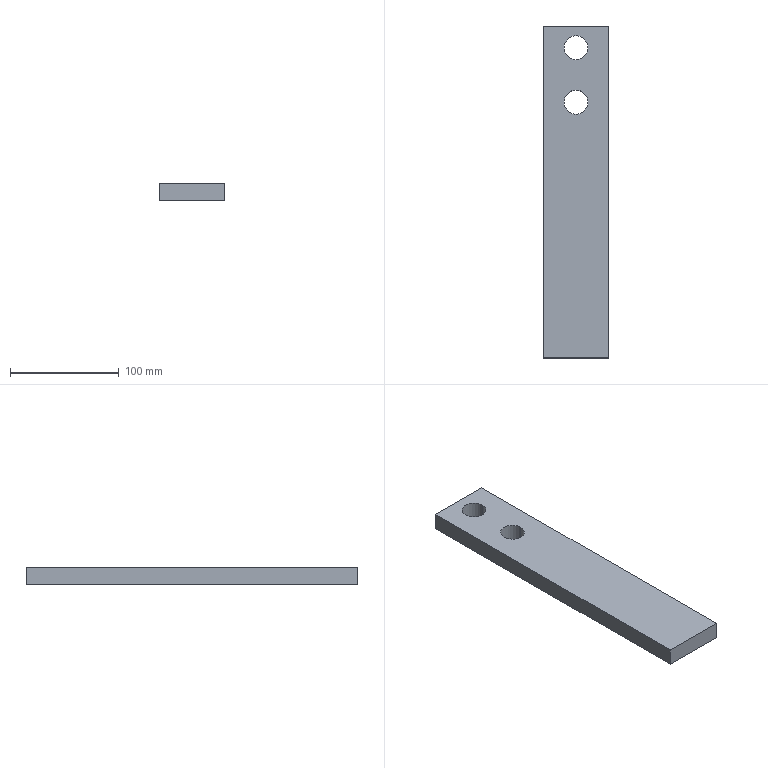Part | SolidWorks | features MirrorStock 1 | 1 solid | 10 faces | box 60 x 305 x 16 mm | volume 280636 mm3 | plane 6 | cylinder 4 | commonest cylinder face diameters 22 x4
STEP:
#1=CARTESIAN_POINT('',(11.,82.5,-8.));
#2=VERTEX_POINT('',#1);
#3=CARTESIAN_POINT('',(-11.,82.5,-8.));
#4=VERTEX_POINT('',#3);
#5=CARTESIAN_POINT('',(0.,82.5,-8.));
#6=DIRECTION('',(0.,0.,1.));
#7=DIRECTION('',(1.,0.,0.));
#8=AXIS2_PLACEMENT_3D('',#5,#6,#7);
#9=CIRCLE('',#8,11.);
#10=EDGE_CURVE('',#2,#4,#9,.T.);
#11=ORIENTED_EDGE('',*,*,#10,.F.);
#12=CARTESIAN_POINT('',(11.,82.5,8.));
#13=VERTEX_POINT('',#12);
#14=CARTESIAN_POINT('',(11.,82.5,-8.));
#15=DIRECTION('',(0.,0.,1.));
#16=VECTOR('',#15,1000.);
#17=LINE('',#14,#16);
#18=EDGE_CURVE('',#2,#13,#17,.T.);
#19=ORIENTED_EDGE('',*,*,#18,.T.);
#20=CARTESIAN_POINT('',(-11.,82.5,8.));
#21=VERTEX_POINT('',#20);
#22=CARTESIAN_POINT('',(0.,82.5,8.));
#23=DIRECTION('',(0.,0.,1.));
#24=DIRECTION('',(1.,0.,0.));
#25=AXIS2_PLACEMENT_3D('',#22,#23,#24);
#26=CIRCLE('',#25,11.);
#27=EDGE_CURVE('',#13,#21,#26,.T.);
#28=ORIENTED_EDGE('',*,*,#27,.T.);
#29=CARTESIAN_POINT('',(-11.,82.5,-8.));
#30=DIRECTION('',(0.,0.,1.));
#31=VECTOR('',#30,1000.);
#32=LINE('',#29,#31);
#33=EDGE_CURVE('',#4,#21,#32,.T.);
#34=ORIENTED_EDGE('',*,*,#33,.F.);
#35=EDGE_LOOP('',(#11,#19,#28,#34));
#36=FACE_OUTER_BOUND('',#35,.T.);
#37=CARTESIAN_POINT('',(0.,82.5,-8.));
#38=DIRECTION('',(0.,0.,1.));
#39=DIRECTION('',(-1.,0.,0.));
#40=AXIS2_PLACEMENT_3D('',#37,#38,#39);
#41=CYLINDRICAL_SURFACE('',#40,11.);
#42=ADVANCED_FACE('',(#36),#41,.F.);
#43=CARTESIAN_POINT('',(11.,132.5,-8.));
#44=VERTEX_POINT('',#43);
#45=CARTESIAN_POINT('',(-11.,132.5,-8.));
#46=VERTEX_POINT('',#45);
#47=CARTESIAN_POINT('',(0.,132.5,-8.));
#48=DIRECTION('',(0.,0.,1.));
#49=DIRECTION('',(1.,0.,0.));
#50=AXIS2_PLACEMENT_3D('',#47,#48,#49);
#51=CIRCLE('',#50,11.);
#52=EDGE_CURVE('',#44,#46,#51,.T.);
#53=ORIENTED_EDGE('',*,*,#52,.F.);
#54=CARTESIAN_POINT('',(11.,132.5,8.));
#55=VERTEX_POINT('',#54);
#56=CARTESIAN_POINT('',(11.,132.5,-8.));
#57=DIRECTION('',(0.,0.,1.));
#58=VECTOR('',#57,1000.);
#59=LINE('',#56,#58);
#60=EDGE_CURVE('',#44,#55,#59,.T.);
#61=ORIENTED_EDGE('',*,*,#60,.T.);
#62=CARTESIAN_POINT('',(-11.,132.5,8.));
#63=VERTEX_POINT('',#62);
#64=CARTESIAN_POINT('',(0.,132.5,8.));
#65=DIRECTION('',(0.,0.,1.));
#66=DIRECTION('',(1.,0.,0.));
#67=AXIS2_PLACEMENT_3D('',#64,#65,#66);
#68=CIRCLE('',#67,11.);
#69=EDGE_CURVE('',#55,#63,#68,.T.);
#70=ORIENTED_EDGE('',*,*,#69,.T.);
#71=CARTESIAN_POINT('',(-11.,132.5,-8.));
#72=DIRECTION('',(0.,0.,1.));
#73=VECTOR('',#72,1000.);
#74=LINE('',#71,#73);
#75=EDGE_CURVE('',#46,#63,#74,.T.);
#76=ORIENTED_EDGE('',*,*,#75,.F.);
#77=EDGE_LOOP('',(#53,#61,#70,#76));
#78=FACE_OUTER_BOUND('',#77,.T.);
#79=CARTESIAN_POINT('',(0.,132.5,-8.));
#80=DIRECTION('',(0.,0.,1.));
#81=DIRECTION('',(-1.,0.,0.));
#82=AXIS2_PLACEMENT_3D('',#79,#80,#81);
#83=CYLINDRICAL_SURFACE('',#82,11.);
#84=ADVANCED_FACE('',(#78),#83,.F.);
#85=CARTESIAN_POINT('',(30.,-152.5,-8.));
#86=VERTEX_POINT('',#85);
#87=CARTESIAN_POINT('',(30.,152.5,-8.));
#88=VERTEX_POINT('',#87);
#89=CARTESIAN_POINT('',(30.,-152.5,-8.));
#90=DIRECTION('',(0.,1.,0.));
#91=VECTOR('',#90,1000.);
#92=LINE('',#89,#91);
#93=EDGE_CURVE('',#86,#88,#92,.T.);
#94=ORIENTED_EDGE('',*,*,#93,.F.);
#95=CARTESIAN_POINT('',(-30.,-152.5,-8.));
#96=VERTEX_POINT('',#95);
#97=CARTESIAN_POINT('',(-30.,-152.5,-8.));
#98=DIRECTION('',(1.,0.,0.));
#99=VECTOR('',#98,1000.);
#100=LINE('',#97,#99);
#101=EDGE_CURVE('',#96,#86,#100,.T.);
#102=ORIENTED_EDGE('',*,*,#101,.F.);
#103=CARTESIAN_POINT('',(-30.,152.5,-8.));
#104=VERTEX_POINT('',#103);
#105=CARTESIAN_POINT('',(-30.,-152.5,-8.));
#106=DIRECTION('',(0.,-1.,0.));
#107=VECTOR('',#106,1000.);
#108=LINE('',#105,#107);
#109=EDGE_CURVE('',#104,#96,#108,.T.);
#110=ORIENTED_EDGE('',*,*,#109,.F.);
#111=CARTESIAN_POINT('',(-30.,152.5,-8.));
#112=DIRECTION('',(-1.,0.,0.));
#113=VECTOR('',#112,1000.);
#114=LINE('',#111,#113);
#115=EDGE_CURVE('',#88,#104,#114,.T.);
#116=ORIENTED_EDGE('',*,*,#115,.F.);
#117=EDGE_LOOP('',(#94,#102,#110,#116));
#118=FACE_OUTER_BOUND('',#117,.T.);
#119=CARTESIAN_POINT('',(0.,132.5,-8.));
#120=DIRECTION('',(0.,0.,1.));
#121=DIRECTION('',(1.,0.,0.));
#122=AXIS2_PLACEMENT_3D('',#119,#120,#121);
#123=CIRCLE('',#122,11.);
#124=EDGE_CURVE('',#46,#44,#123,.T.);
#125=ORIENTED_EDGE('',*,*,#124,.T.);
#126=ORIENTED_EDGE('',*,*,#52,.T.);
#127=EDGE_LOOP('',(#125,#126));
#128=FACE_BOUND('',#127,.T.);
#129=CARTESIAN_POINT('',(0.,82.5,-8.));
#130=DIRECTION('',(0.,0.,1.));
#131=DIRECTION('',(1.,0.,0.));
#132=AXIS2_PLACEMENT_3D('',#129,#130,#131);
#133=CIRCLE('',#132,11.);
#134=EDGE_CURVE('',#4,#2,#133,.T.);
#135=ORIENTED_EDGE('',*,*,#134,.T.);
#136=ORIENTED_EDGE('',*,*,#10,.T.);
#137=EDGE_LOOP('',(#135,#136));
#138=FACE_BOUND('',#137,.T.);
#139=CARTESIAN_POINT('',(0.,0.,-8.));
#140=DIRECTION('',(0.,0.,1.));
#141=DIRECTION('',(-1.,0.,0.));
#142=AXIS2_PLACEMENT_3D('',#139,#140,#141);
#143=PLANE('',#142);
#144=ADVANCED_FACE('',(#118,#128,#138),#143,.F.);
#145=CARTESIAN_POINT('',(0.,132.5,8.));
#146=DIRECTION('',(0.,0.,1.));
#147=DIRECTION('',(1.,0.,0.));
#148=AXIS2_PLACEMENT_3D('',#145,#146,#147);
#149=CIRCLE('',#148,11.);
#150=EDGE_CURVE('',#63,#55,#149,.T.);
#151=ORIENTED_EDGE('',*,*,#150,.F.);
#152=ORIENTED_EDGE('',*,*,#69,.F.);
#153=EDGE_LOOP('',(#151,#152));
#154=FACE_BOUND('',#153,.T.);
#155=CARTESIAN_POINT('',(30.,-152.5,8.));
#156=VERTEX_POINT('',#155);
#157=CARTESIAN_POINT('',(30.,152.5,8.));
#158=VERTEX_POINT('',#157);
#159=CARTESIAN_POINT('',(30.,-152.5,8.));
#160=DIRECTION('',(0.,1.,0.));
#161=VECTOR('',#160,1000.);
#162=LINE('',#159,#161);
#163=EDGE_CURVE('',#156,#158,#162,.T.);
#164=ORIENTED_EDGE('',*,*,#163,.T.);
#165=CARTESIAN_POINT('',(-30.,152.5,8.));
#166=VERTEX_POINT('',#165);
#167=CARTESIAN_POINT('',(-30.,152.5,8.));
#168=DIRECTION('',(-1.,0.,0.));
#169=VECTOR('',#168,1000.);
#170=LINE('',#167,#169);
#171=EDGE_CURVE('',#158,#166,#170,.T.);
#172=ORIENTED_EDGE('',*,*,#171,.T.);
#173=CARTESIAN_POINT('',(-30.,-152.5,8.));
#174=VERTEX_POINT('',#173);
#175=CARTESIAN_POINT('',(-30.,-152.5,8.));
#176=DIRECTION('',(0.,-1.,0.));
#177=VECTOR('',#176,1000.);
#178=LINE('',#175,#177);
#179=EDGE_CURVE('',#166,#174,#178,.T.);
#180=ORIENTED_EDGE('',*,*,#179,.T.);
#181=CARTESIAN_POINT('',(-30.,-152.5,8.));
#182=DIRECTION('',(1.,0.,0.));
#183=VECTOR('',#182,1000.);
#184=LINE('',#181,#183);
#185=EDGE_CURVE('',#174,#156,#184,.T.);
#186=ORIENTED_EDGE('',*,*,#185,.T.);
#187=EDGE_LOOP('',(#164,#172,#180,#186));
#188=FACE_OUTER_BOUND('',#187,.T.);
#189=CARTESIAN_POINT('',(0.,82.5,8.));
#190=DIRECTION('',(0.,0.,1.));
#191=DIRECTION('',(1.,0.,0.));
#192=AXIS2_PLACEMENT_3D('',#189,#190,#191);
#193=CIRCLE('',#192,11.);
#194=EDGE_CURVE('',#21,#13,#193,.T.);
#195=ORIENTED_EDGE('',*,*,#194,.F.);
#196=ORIENTED_EDGE('',*,*,#27,.F.);
#197=EDGE_LOOP('',(#195,#196));
#198=FACE_BOUND('',#197,.T.);
#199=CARTESIAN_POINT('',(0.,0.,8.));
#200=DIRECTION('',(0.,0.,1.));
#201=DIRECTION('',(-1.,0.,0.));
#202=AXIS2_PLACEMENT_3D('',#199,#200,#201);
#203=PLANE('',#202);
#204=ADVANCED_FACE('',(#154,#188,#198),#203,.T.);
#205=ORIENTED_EDGE('',*,*,#163,.F.);
#206=CARTESIAN_POINT('',(30.,-152.5,-8.));
#207=DIRECTION('',(0.,0.,1.));
#208=VECTOR('',#207,1000.);
#209=LINE('',#206,#208);
#210=EDGE_CURVE('',#86,#156,#209,.T.);
#211=ORIENTED_EDGE('',*,*,#210,.F.);
#212=ORIENTED_EDGE('',*,*,#93,.T.);
#213=CARTESIAN_POINT('',(30.,152.5,-8.));
#214=DIRECTION('',(0.,0.,1.));
#215=VECTOR('',#214,1000.);
#216=LINE('',#213,#215);
#217=EDGE_CURVE('',#88,#158,#216,.T.);
#218=ORIENTED_EDGE('',*,*,#217,.T.);
#219=EDGE_LOOP('',(#205,#211,#212,#218));
#220=FACE_OUTER_BOUND('',#219,.T.);
#221=CARTESIAN_POINT('',(30.,-152.5,-8.));
#222=DIRECTION('',(-1.,0.,0.));
#223=DIRECTION('',(0.,0.,-1.));
#224=AXIS2_PLACEMENT_3D('',#221,#222,#223);
#225=PLANE('',#224);
#226=ADVANCED_FACE('',(#220),#225,.F.);
#227=ORIENTED_EDGE('',*,*,#171,.F.);
#228=ORIENTED_EDGE('',*,*,#217,.F.);
#229=ORIENTED_EDGE('',*,*,#115,.T.);
#230=CARTESIAN_POINT('',(-30.,152.5,-8.));
#231=DIRECTION('',(0.,0.,1.));
#232=VECTOR('',#231,1000.);
#233=LINE('',#230,#232);
#234=EDGE_CURVE('',#104,#166,#233,.T.);
#235=ORIENTED_EDGE('',*,*,#234,.T.);
#236=EDGE_LOOP('',(#227,#228,#229,#235));
#237=FACE_OUTER_BOUND('',#236,.T.);
#238=CARTESIAN_POINT('',(-30.,152.5,-8.));
#239=DIRECTION('',(0.,-1.,0.));
#240=DIRECTION('',(0.,0.,1.));
#241=AXIS2_PLACEMENT_3D('',#238,#239,#240);
#242=PLANE('',#241);
#243=ADVANCED_FACE('',(#237),#242,.F.);
#244=ORIENTED_EDGE('',*,*,#179,.F.);
#245=ORIENTED_EDGE('',*,*,#234,.F.);
#246=ORIENTED_EDGE('',*,*,#109,.T.);
#247=CARTESIAN_POINT('',(-30.,-152.5,-8.));
#248=DIRECTION('',(0.,0.,1.));
#249=VECTOR('',#248,1000.);
#250=LINE('',#247,#249);
#251=EDGE_CURVE('',#96,#174,#250,.T.);
#252=ORIENTED_EDGE('',*,*,#251,.T.);
#253=EDGE_LOOP('',(#244,#245,#246,#252));
#254=FACE_OUTER_BOUND('',#253,.T.);
#255=CARTESIAN_POINT('',(-30.,-152.5,-8.));
#256=DIRECTION('',(1.,0.,0.));
#257=DIRECTION('',(0.,0.,1.));
#258=AXIS2_PLACEMENT_3D('',#255,#256,#257);
#259=PLANE('',#258);
#260=ADVANCED_FACE('',(#254),#259,.F.);
#261=ORIENTED_EDGE('',*,*,#185,.F.);
#262=ORIENTED_EDGE('',*,*,#251,.F.);
#263=ORIENTED_EDGE('',*,*,#101,.T.);
#264=ORIENTED_EDGE('',*,*,#210,.T.);
#265=EDGE_LOOP('',(#261,#262,#263,#264));
#266=FACE_OUTER_BOUND('',#265,.T.);
#267=CARTESIAN_POINT('',(-30.,-152.5,-8.));
#268=DIRECTION('',(0.,1.,0.));
#269=DIRECTION('',(0.,0.,-1.));
#270=AXIS2_PLACEMENT_3D('',#267,#268,#269);
#271=PLANE('',#270);
#272=ADVANCED_FACE('',(#266),#271,.F.);
#273=ORIENTED_EDGE('',*,*,#60,.F.);
#274=ORIENTED_EDGE('',*,*,#124,.F.);
#275=ORIENTED_EDGE('',*,*,#75,.T.);
#276=ORIENTED_EDGE('',*,*,#150,.T.);
#277=EDGE_LOOP('',(#273,#274,#275,#276));
#278=FACE_OUTER_BOUND('',#277,.T.);
#279=CARTESIAN_POINT('',(0.,132.5,-8.));
#280=DIRECTION('',(0.,0.,1.));
#281=DIRECTION('',(-1.,0.,0.));
#282=AXIS2_PLACEMENT_3D('',#279,#280,#281);
#283=CYLINDRICAL_SURFACE('',#282,11.);
#284=ADVANCED_FACE('',(#278),#283,.F.);
#285=ORIENTED_EDGE('',*,*,#18,.F.);
#286=ORIENTED_EDGE('',*,*,#134,.F.);
#287=ORIENTED_EDGE('',*,*,#33,.T.);
#288=ORIENTED_EDGE('',*,*,#194,.T.);
#289=EDGE_LOOP('',(#285,#286,#287,#288));
#290=FACE_OUTER_BOUND('',#289,.T.);
#291=CARTESIAN_POINT('',(0.,82.5,-8.));
#292=DIRECTION('',(0.,0.,1.));
#293=DIRECTION('',(-1.,0.,0.));
#294=AXIS2_PLACEMENT_3D('',#291,#292,#293);
#295=CYLINDRICAL_SURFACE('',#294,11.);
#296=ADVANCED_FACE('',(#290),#295,.F.);
#297=CLOSED_SHELL('',(#42,#84,#144,#204,#226,#243,#260,#272,#284,#296));
#298=MANIFOLD_SOLID_BREP('',#297);
#299=CARTESIAN_POINT('',(0.,0.,0.));
#300=DIRECTION('',(0.,0.,1.));
#301=DIRECTION('',(1.,0.,0.));
#302=AXIS2_PLACEMENT_3D('',#299,#300,#301);
#303=(LENGTH_UNIT()NAMED_UNIT(*)SI_UNIT(.MILLI.,.METRE.));
#304=UNCERTAINTY_MEASURE_WITH_UNIT(LENGTH_MEASURE(0.00001),#303,'','');
#305=(NAMED_UNIT(*)PLANE_ANGLE_UNIT()SI_UNIT($,.RADIAN.));
#306=(NAMED_UNIT(*)SI_UNIT($,.STERADIAN.)SOLID_ANGLE_UNIT());
#307=(GEOMETRIC_REPRESENTATION_CONTEXT(3)GLOBAL_UNCERTAINTY_ASSIGNED_CONTEXT((#304))GLOBAL_UNIT_ASSIGNED_CONTEXT((#303,#305,#306))REPRESENTATION_CONTEXT('',''));
#308=ADVANCED_BREP_SHAPE_REPRESENTATION('',(#298,#302),#307);